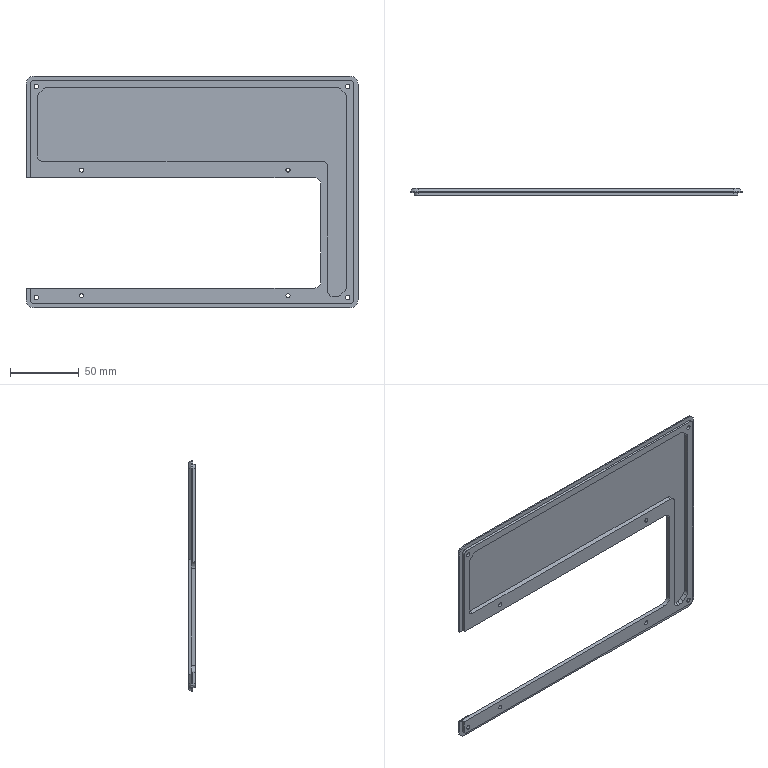Part | 1 solid | 80 faces | box 242 x 5 x 169 mm | volume 56011 mm3 | plane 39 | cylinder 33 | cone 8 | commonest cylinder face diameters 8 x15 3 x4 3.2 x4 5.6 x4 12 x4 10 x2